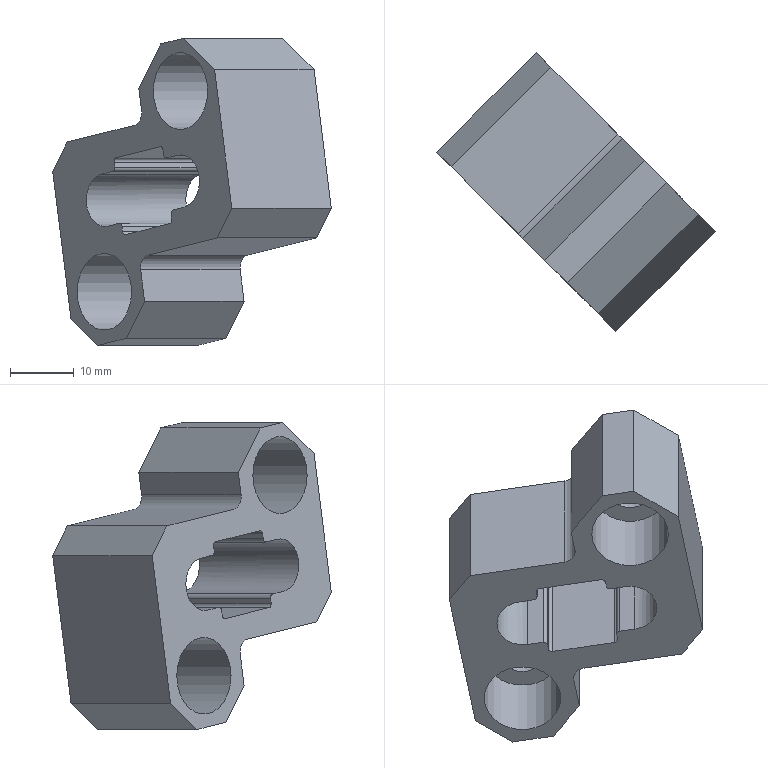Part | STEP file | gslz 2016.10.28-13_id1382_x_t | 1 solid | 48 faces | box 43.55 x 43.55 x 48.008 mm | volume 15438 mm3 | plane 19 | cylinder 16 | spline 11 | other 2 | commonest cylinder face diameters 1.2 x8 4 x2 6 x2 6.8 x2 12 x2